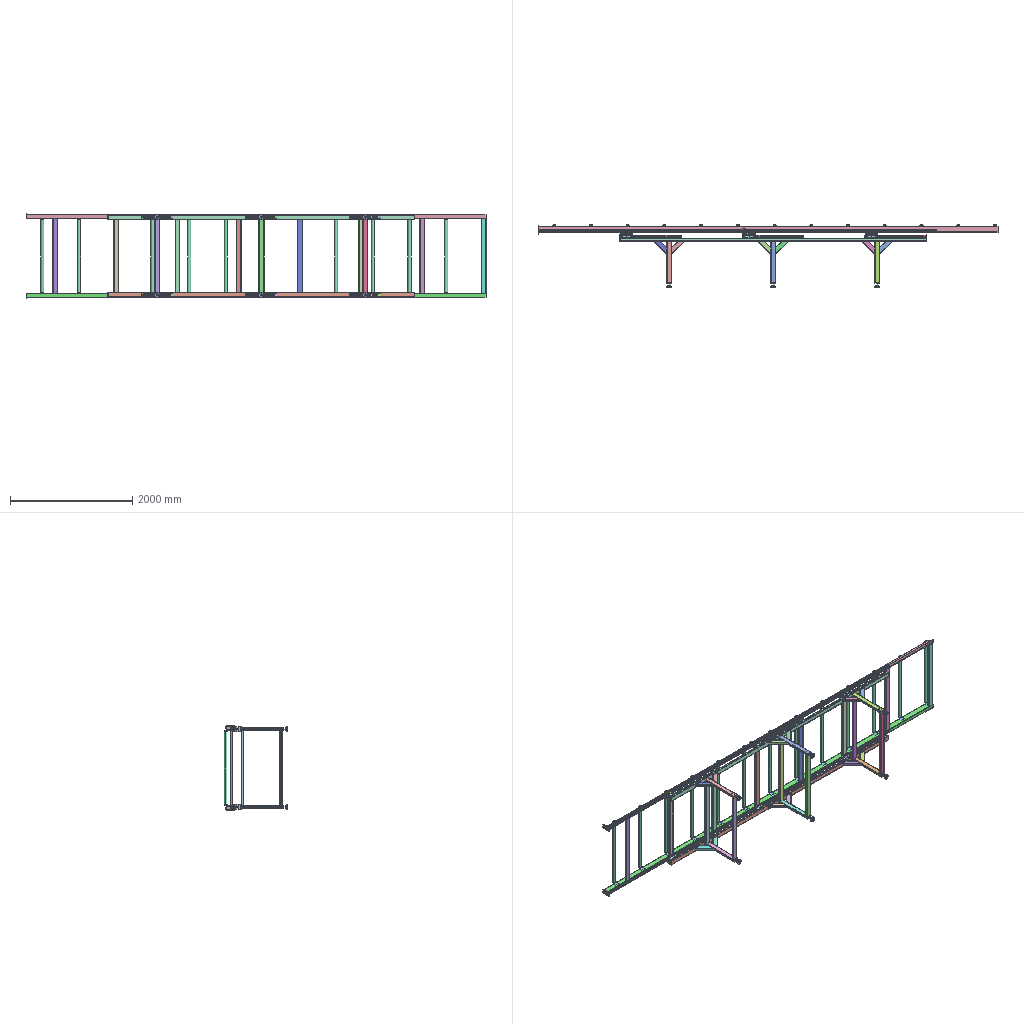Assembly | SolidWorks | 17 different items | 90 placed | box 7516 x 1042 x 1380 mm
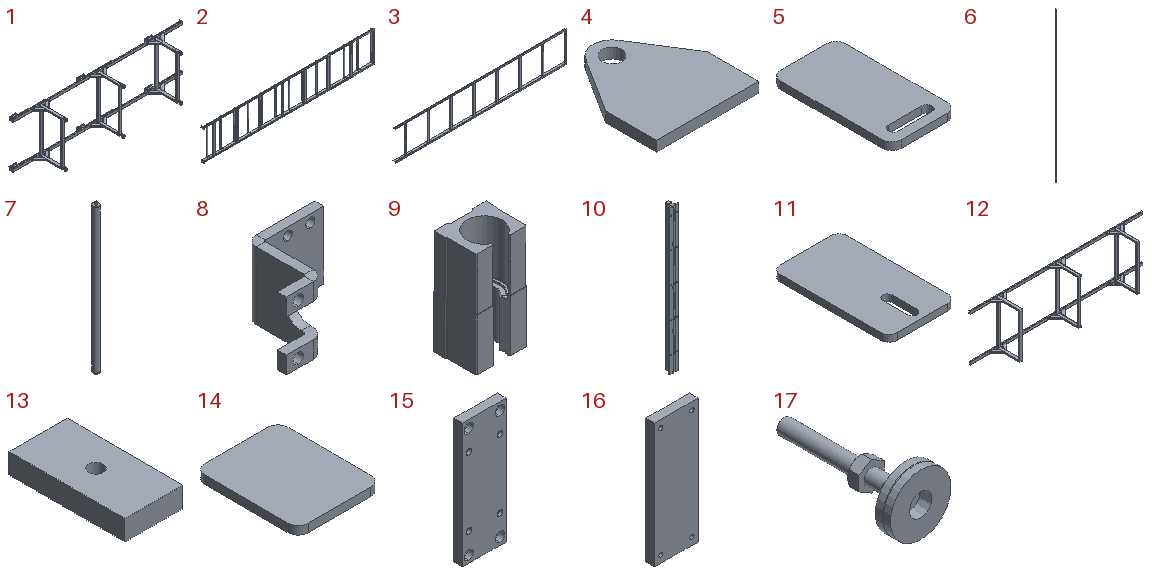Parts list (item | name | quantity | parent item | size | volume | features):
1 | (subassembly) | x1 | - | - | 30307292 mm3 | features ReferencePattern 16, LocalLPattern 1
2 | (subassembly) | x1 | - | 7516 x 170 x 1380 mm | 38650650 mm3 | features ReferencePattern 36, LocalLPattern 1
3 | - | x1 | in 2 | 7500 x 100 x 1356 mm | 20928649 mm3 | features WeldMemberFeat 3, 3DProfileFeature 2, WeldmentFeature 1
4 | - | x26 | in 2 | 80 x 90 x 8 mm | 43119 mm3 | features Extrusion 1
5 | - | x2 | in 2 | 70 x 130 x 8 mm | 68185 mm3 | features Extrusion 1, ICE 1
6 | - | x2 | in 2 | 45 x 37 x 6500 mm | 4217022 mm3 | features Chamfer 1, Extrusion 1, ICE 1, LPattern 1, MirrorPattern 1, RevCut 1
7 | - | x13 | in 2 | 50 x 50 x 1240 mm | 604574 mm3 | features Chamfer 2, ICE 2, RevCut 1, Revolution 1
8 | - | x1 | - | 65 x 46 x 45 mm | 21673 mm3 | features ICE 3, FlatPattern 1, SMBaseFlange 1, SheetMetal 1
9 | - | x6 | in 1 | 70 x 56 x 140 mm | 330952 mm3 | features Fillet 2, ICE 2, RevCut 2, Extrusion 1, SketchPattern 1
10 | - | x6 | in 1 | 60 x 52 x 1000 mm | 1438774 mm3 | features RevCut 2, Chamfer 1, CurvePattern 1, Extrusion 1, ICE 1, MirrorPattern 1
11 | - | x2 | in 2 | 80 x 140 x 8 mm | 85513 mm3 | features Extrusion 1, ICE 1
12 | - | x1 | in 1 | 5000 x 710 x 1350 mm | 15935938 mm3 | features WeldCornerFeat 6, 3DProfileFeature 1, WeldMemberFeat 1, WeldmentFeature 1
13 | - | x6 | in 1 | 40 x 80 x 14 mm | 43700 mm3 | features Extrusion 1, HoleWzd 1
14 | - | x4 | in 1 | 80 x 100 x 8 mm | 63313 mm3 | features Extrusion 1
15 | - | x6 | in 1 | 70 x 14 x 200 mm | 180732 mm3 | features HoleWzd 2, Extrusion 1
16 | - | x6 | in 1 | 70 x 14 x 200 mm | 193966 mm3 | features HoleWzd 2, Extrusion 1
17 | - | x6 | in 1 | 80 x 181 x 80 mm | 164891 mm3 | features ICE 2, RevCut 2, Chamfer 1, Revolution 1
Mates (type | each side: item.copy, entity, surface, feature):
In the top assembly
Width | assembly face | assembly face | assembly face
Coincident | 16.1 face plane Boss-Extrude1 | 3.1 face plane Gb/t9788-1988 hot-rolled unequal angle 10/6.3 D=6(3)
Width | 12.1 face plane 80 X 40 X 3 - missing(1) | 12.1 face plane 80 X 40 X 3 - missing(1) | 3.1 face plane Gb/t9788-1988 hot-rolled unequal angle 10/6.3 D=6(3) | 3.1 face plane Gb/t9788-1988 hot-rolled unequal angle 10/6.3 D=6(2)
DistanceDim | 11.1 face plane Boss-Extrude1 | 16.1 face plane Boss-Extrude1
In subassembly 2
Coincident | 3.2 face plane Gb/t9788-1988 hot-rolled unequal angle 10/6.3 D=6(2) | 4.1 face plane Boss-Extrude1
DistanceDim | 4.1 face plane Boss-Extrude1 | 3.2 face plane Gb/t9788-1988 hot-rolled unequal angle 10/6.3 D=6(2)
DistanceDim | 3.2 face plane Gb/t9788-1988 hot-rolled unequal angle 10/6.3 D=6(2) | 4.1 face plane Boss-Extrude1
Coincident | 3.2 face plane Gb/t9788-1988 hot-rolled unequal angle 10/6.3 D=6(3) | 4.2 face plane Boss-Extrude1
Concentric | 4.1 face cylinder Boss-Extrude1 | 4.2 face cylinder Boss-Extrude1
Coincident | 4.1 face plane Boss-Extrude1 | 4.2 face plane Boss-Extrude1
Coincident | 3.2 face plane Gb/t9788-1988 hot-rolled unequal angle 10/6.3 D=6(3) | 6.1 face plane Boss-Extrude1 | 3 times
Coincident | 3.2 face plane Gb/t9788-1988 hot-rolled unequal angle 10/6.3 D=6(2) | 6.2 face plane Boss-Extrude1 | 3 times
Coincident | 3.2 face plane Gb/t9788-1988 hot-rolled unequal angle 10/6.3 D=6(3) | 5.1 face plane Boss-Extrude1 | 2 times
DistanceDim | 3.2 face plane Gb/t9788-1988 hot-rolled unequal angle 10/6.3 D=6(3) | 5.1 face plane Boss-Extrude1
Coincident | 5.1 face plane Boss-Extrude1 | 5.2 face plane Boss-Extrude1
Coincident | 3.2 face plane Gb/t9788-1988 hot-rolled unequal angle 10/6.3 D=6(2) | 5.2 face plane Boss-Extrude1 | 2 times
Concentric | 4.1 face cylinder Boss-Extrude1 | 7.1 face cylinder Revolve1
DistanceDim | 7.1 face plane Revolve1 | 4.1 face plane Boss-Extrude1
Coincident | 5.1 face plane Boss-Extrude1 | 11.2 face plane Boss-Extrude1 | 2 times
DistanceDim | 11.2 face plane Boss-Extrude1 | 5.1 face plane Boss-Extrude1
Coincident | 5.2 face plane Boss-Extrude1 | 11.3 face plane Boss-Extrude1 | 2 times
DistanceDim | 11.3 face plane Boss-Extrude1 | 5.2 face plane Boss-Extrude1
In subassembly 1
Coincident | 12.2 face plane 80 X 40 X 3 - missing(1) | 13.1 face plane Boss-Extrude1 | 3 times
Coincident | 13.1 face plane Boss-Extrude1 | 17.1 face plane Boss-Extrude2
Concentric | 13.1 face cylinder Boss-Extrude1 | 17.1 face cylinder Revolve1
Coincident | 12.2 face plane 80 X 40 X 3 - missing(1) | 13.2 face plane Boss-Extrude1 | 3 times
Coincident | 13.2 face plane Boss-Extrude1 | 17.2 face plane Boss-Extrude2
Concentric | 13.2 face cylinder Boss-Extrude1 | 17.2 face cylinder Revolve1
Coincident | 12.2 face plane 80 X 40 X 3 - missing(1) | 13.3 face plane Boss-Extrude1 | 3 times
Coincident | 17.3 face plane Boss-Extrude2 | 13.3 face plane Boss-Extrude1
Concentric | 17.3 face cylinder Revolve1 | 13.3 face cylinder Boss-Extrude1
Coincident | 12.2 face plane 80 X 40 X 3 - missing(1) | 13.4 face plane Boss-Extrude1 | 3 times
Coincident | 13.4 face plane Boss-Extrude1 | 17.4 face plane Boss-Extrude2
Concentric | 13.4 face cylinder Boss-Extrude1 | 17.4 face cylinder Revolve1
Coincident | 12.2 face plane 80 X 40 X 3 - missing(1) | 13.5 face plane Boss-Extrude1 | 3 times
Coincident | 13.5 face plane Boss-Extrude1 | 17.5 face plane Boss-Extrude2
Concentric | 13.5 face cylinder Boss-Extrude1 | 17.5 face cylinder Revolve1
Coincident | 12.2 face plane 80 X 40 X 3 - missing(1) | 13.6 face plane Boss-Extrude1 | 3 times
Coincident | 13.6 face plane Boss-Extrude1 | 17.6 face plane Boss-Extrude2
Concentric | 13.6 face cylinder Boss-Extrude1 | 17.6 face cylinder Revolve1
Coincident | 12.2 face plane 80 X 40 X 3 - missing(1) | 14.1 face plane Boss-Extrude1 | 3 times
Coincident | 12.2 face plane 80 X 40 X 3 - missing(1) | 14.2 face plane Boss-Extrude1 | 3 times
Coincident | 12.2 face plane 80 X 40 X 3 - missing(1) | 14.3 face plane Boss-Extrude1 | 3 times
Coincident | 12.2 face plane 80 X 40 X 3 - missing(1) | 14.4 face plane Boss-Extrude1 | 3 times
Coincident | 12.2 face plane 80 X 40 X 3 - missing(1) | 10.1 face plane Boss-Extrude1
Coincident | 14.3 face plane Boss-Extrude1 | 10.1 face plane Boss-Extrude1
DistanceDim | 10.1 face plane Boss-Extrude1 | 12.2 face plane 80 X 40 X 3 - missing(1)
Coincident | 12.2 face plane 80 X 40 X 3 - missing(1) | 10.2 face plane Boss-Extrude1
Coincident | 14.4 face plane Boss-Extrude1 | 10.2 face plane Boss-Extrude1
DistanceDim | 10.2 face plane Boss-Extrude1 | 12.2 face plane 80 X 40 X 3 - missing(1)
Concentric | 10.1 face cylinder Boss-Extrude2 | 9.1 face cylinder Boss-Extrude1
Concentric | 10.2 face cylinder Boss-Extrude2 | 9.2 face cylinder Boss-Extrude1
Coincident | 9.1 face plane Boss-Extrude1 | 9.2 face plane Boss-Extrude1 | 2 times
Coincident | 9.1 face plane Boss-Extrude1 | 15.1 face plane Boss-Extrude1 | 2 times
DistanceDim | 15.1 face plane Boss-Extrude1 | 9.1 face plane Boss-Extrude1
Coincident | 9.2 face plane Boss-Extrude1 | 15.2 face plane Boss-Extrude1
Coincident | 15.1 face plane Boss-Extrude1 | 15.2 face plane Boss-Extrude1 | 2 times
Coincident | 15.2 face plane Boss-Extrude1 | 16.2 face plane Boss-Extrude1
Concentric | 15.2 face cylinder Hole size (%based on) socket head cap screw type2 | 16.2 face cylinder M8 Tapped Hole1 | 2 times
Coincident | 15.1 face plane Boss-Extrude1 | 16.3 face plane Boss-Extrude1
Concentric | 15.1 face cylinder Hole size (%based on) socket head cap screw type2 | 16.3 face cylinder M8 Tapped Hole1 | 2 times